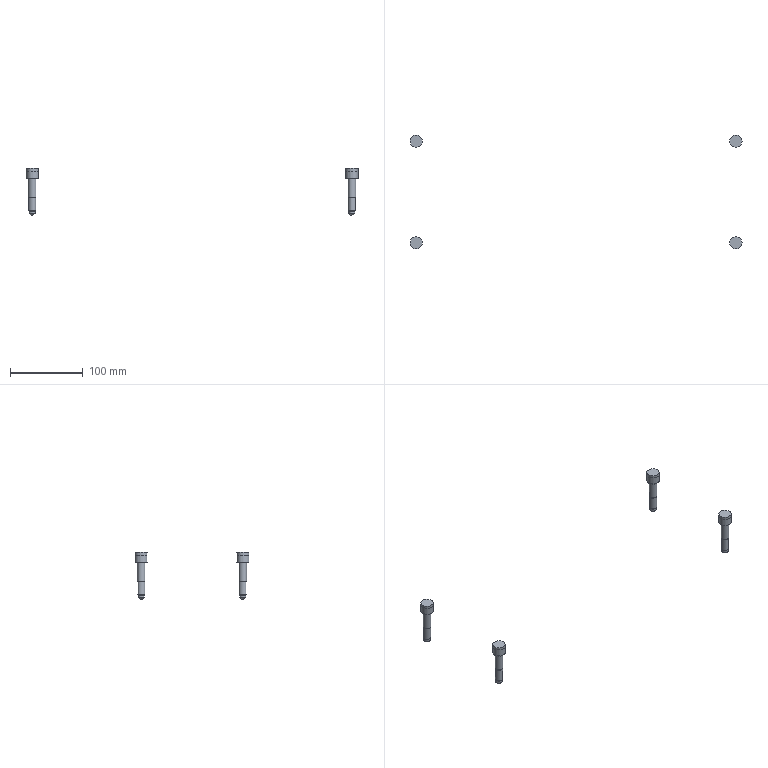Part | NX | features BREP 2 | 8 solids | 84 faces | box 457 x 157 x 65.231 mm | volume 47767 mm3 | plane 56 | cylinder 20 | cone 8 | commonest cylinder face diameters 8.5 x4 10 x4 10.5 x4 16 x4 17 x4